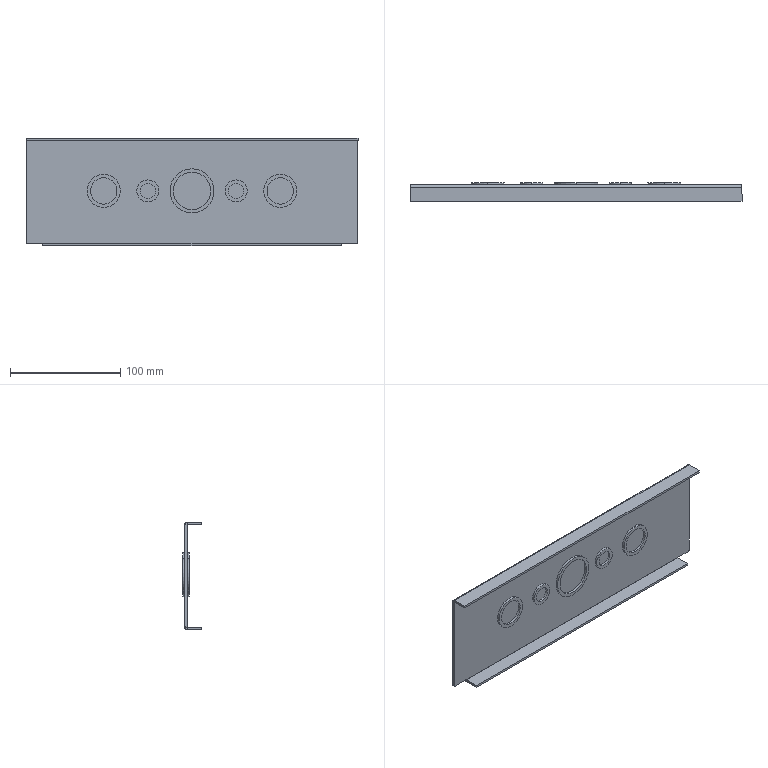Part | SolidWorks | features EdgeFlange 2, ICE 2, Fillet 1, FlatPattern 1, SMBaseFlange 1, SheetMetal 1 | 1 solid | 92 faces | box 300.8 x 17 x 97.6 mm | volume 77629 mm3 | cylinder 46 | plane 46 | commonest cylinder face diameters 14 x8 20 x8 24 x8 30 x8 34 x4 40 x4